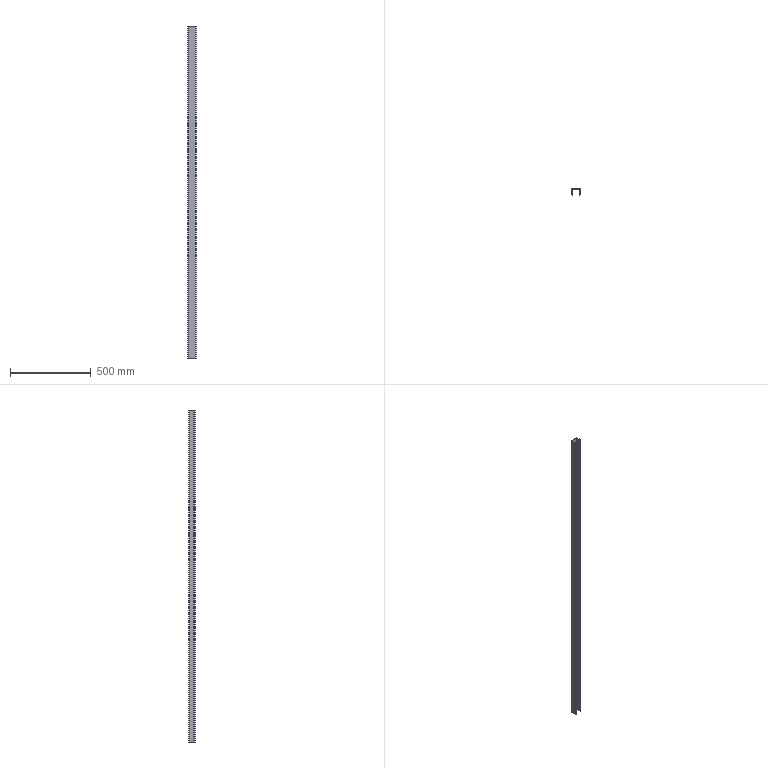Part | STEP file | 31E-01029QY25 | 1 solid | 28 faces | box 50 x 38.192 x 2050 mm | volume 337512 mm3 | plane 16 | cylinder 12 | commonest cylinder face diameters 1 x4 2 x4 4 x2 26 x2
STEP:
#1=CARTESIAN_POINT('',(27.993,8.298,1025.));
#2=VERTEX_POINT('',#1);
#3=CARTESIAN_POINT('',(32.281,3.187,1025.));
#4=VERTEX_POINT('',#3);
#5=CARTESIAN_POINT('',(30.137,5.743,1025.));
#6=DIRECTION('',(0.6428,-0.766,0.));
#7=VECTOR('',#6,1.);
#8=LINE('',#5,#7);
#9=EDGE_CURVE('',#2,#4,#8,.T.);
#10=ORIENTED_EDGE('',*,*,#9,.F.);
#11=CARTESIAN_POINT('',(27.993,8.298,-1025.));
#12=VERTEX_POINT('',#11);
#13=CARTESIAN_POINT('',(27.993,8.298,0.));
#14=DIRECTION('',(0.,0.,-1.));
#15=VECTOR('',#14,1.);
#16=LINE('',#13,#15);
#17=EDGE_CURVE('',#2,#12,#16,.T.);
#18=ORIENTED_EDGE('',*,*,#17,.T.);
#19=CARTESIAN_POINT('',(32.281,3.187,-1025.));
#20=VERTEX_POINT('',#19);
#21=CARTESIAN_POINT('',(30.137,5.743,-1025.));
#22=DIRECTION('',(0.6428,-0.766,0.));
#23=VECTOR('',#22,1.);
#24=LINE('',#21,#23);
#25=EDGE_CURVE('',#12,#20,#24,.T.);
#26=ORIENTED_EDGE('',*,*,#25,.T.);
#27=CARTESIAN_POINT('',(32.281,3.187,0.));
#28=DIRECTION('',(0.,0.,-1.));
#29=VECTOR('',#28,1.);
#30=LINE('',#27,#29);
#31=EDGE_CURVE('',#4,#20,#30,.T.);
#32=ORIENTED_EDGE('',*,*,#31,.F.);
#33=EDGE_LOOP('',(#10,#18,#26,#32));
#34=FACE_OUTER_BOUND('',#33,.T.);
#35=CARTESIAN_POINT('',(27.525,8.856,1025.));
#36=DIRECTION('',(0.766,0.6428,0.));
#37=DIRECTION('',(-0.6428,0.766,0.));
#38=AXIS2_PLACEMENT_3D('',#35,#36,#37);
#39=PLANE('',#38);
#40=ADVANCED_FACE('',(#34),#39,.F.);
#41=CARTESIAN_POINT('',(76.525,38.856,1025.));
#42=VERTEX_POINT('',#41);
#43=CARTESIAN_POINT('',(28.525,38.856,1025.));
#44=VERTEX_POINT('',#43);
#45=CARTESIAN_POINT('',(52.525,38.856,1025.));
#46=DIRECTION('',(-1.,0.,0.));
#47=VECTOR('',#46,1.);
#48=LINE('',#45,#47);
#49=EDGE_CURVE('',#42,#44,#48,.T.);
#50=ORIENTED_EDGE('',*,*,#49,.T.);
#51=CARTESIAN_POINT('',(27.525,37.856,1025.));
#52=VERTEX_POINT('',#51);
#53=CARTESIAN_POINT('',(28.525,37.856,1025.));
#54=DIRECTION('',(0.,0.,1.));
#55=AXIS2_PLACEMENT_3D('',#53,#54,$);
#56=CIRCLE('',#55,1.);
#57=EDGE_CURVE('',#44,#52,#56,.T.);
#58=ORIENTED_EDGE('',*,*,#57,.T.);
#59=CARTESIAN_POINT('',(27.525,9.584,1025.));
#60=VERTEX_POINT('',#59);
#61=CARTESIAN_POINT('',(27.525,23.72,1025.));
#62=DIRECTION('',(0.,-1.,0.));
#63=VECTOR('',#62,1.);
#64=LINE('',#61,#63);
#65=EDGE_CURVE('',#52,#60,#64,.T.);
#66=ORIENTED_EDGE('',*,*,#65,.T.);
#67=CARTESIAN_POINT('',(29.525,9.584,1025.));
#68=DIRECTION('',(0.,0.,1.));
#69=AXIS2_PLACEMENT_3D('',#67,#68,$);
#70=CIRCLE('',#69,2.);
#71=EDGE_CURVE('',#60,#2,#70,.T.);
#72=ORIENTED_EDGE('',*,*,#71,.T.);
#73=ORIENTED_EDGE('',*,*,#9,.T.);
#74=CARTESIAN_POINT('',(28.342,2.493,1025.));
#75=VERTEX_POINT('',#74);
#76=CARTESIAN_POINT('',(30.312,2.84,1025.));
#77=DIRECTION('',(-0.9848,-0.1736,0.));
#78=VECTOR('',#77,1.);
#79=LINE('',#76,#78);
#80=EDGE_CURVE('',#4,#75,#79,.T.);
#81=ORIENTED_EDGE('',*,*,#80,.T.);
#82=CARTESIAN_POINT('',(32.653,0.6877,1025.));
#83=VERTEX_POINT('',#82);
#84=CARTESIAN_POINT('',(35.437,13.386,1025.));
#85=DIRECTION('',(0.,0.,1.));
#86=AXIS2_PLACEMENT_3D('',#84,#85,$);
#87=CIRCLE('',#86,13.);
#88=EDGE_CURVE('',#75,#83,#87,.T.);
#89=ORIENTED_EDGE('',*,*,#88,.T.);
#90=CARTESIAN_POINT('',(33.867,1.665,1025.));
#91=VERTEX_POINT('',#90);
#92=CARTESIAN_POINT('',(32.867,1.665,1025.));
#93=DIRECTION('',(0.,0.,1.));
#94=AXIS2_PLACEMENT_3D('',#92,#93,$);
#95=CIRCLE('',#94,1.);
#96=EDGE_CURVE('',#83,#91,#95,.T.);
#97=ORIENTED_EDGE('',*,*,#96,.T.);
#98=CARTESIAN_POINT('',(33.867,2.983,1025.));
#99=VERTEX_POINT('',#98);
#100=CARTESIAN_POINT('',(33.867,2.324,1025.));
#101=DIRECTION('',(0.,1.,0.));
#102=VECTOR('',#101,1.);
#103=LINE('',#100,#102);
#104=EDGE_CURVE('',#91,#99,#103,.T.);
#105=ORIENTED_EDGE('',*,*,#104,.T.);
#106=CARTESIAN_POINT('',(33.75,3.304,1025.));
#107=VERTEX_POINT('',#106);
#108=CARTESIAN_POINT('',(33.367,2.983,1025.));
#109=DIRECTION('',(0.,0.,1.));
#110=AXIS2_PLACEMENT_3D('',#108,#109,$);
#111=CIRCLE('',#110,0.5);
#112=EDGE_CURVE('',#99,#107,#111,.T.);
#113=ORIENTED_EDGE('',*,*,#112,.T.);
#114=CARTESIAN_POINT('',(28.725,9.293,1025.));
#115=VERTEX_POINT('',#114);
#116=CARTESIAN_POINT('',(31.237,6.298,1025.));
#117=DIRECTION('',(-0.6428,0.766,0.));
#118=VECTOR('',#117,1.);
#119=LINE('',#116,#118);
#120=EDGE_CURVE('',#107,#115,#119,.T.);
#121=ORIENTED_EDGE('',*,*,#120,.T.);
#122=CARTESIAN_POINT('',(28.725,37.156,1025.));
#123=VERTEX_POINT('',#122);
#124=CARTESIAN_POINT('',(28.725,23.225,1025.));
#125=DIRECTION('',(0.,1.,0.));
#126=VECTOR('',#125,1.);
#127=LINE('',#124,#126);
#128=EDGE_CURVE('',#115,#123,#127,.T.);
#129=ORIENTED_EDGE('',*,*,#128,.T.);
#130=CARTESIAN_POINT('',(29.225,37.656,1025.));
#131=VERTEX_POINT('',#130);
#132=CARTESIAN_POINT('',(28.725,37.156,1025.));
#133=CARTESIAN_POINT('',(28.725,37.219,1025.));
#134=CARTESIAN_POINT('',(28.735,37.282,1025.));
#135=CARTESIAN_POINT('',(28.754,37.343,1025.));
#136=CARTESIAN_POINT('',(28.812,37.456,1025.));
#137=CARTESIAN_POINT('',(28.902,37.546,1025.));
#138=CARTESIAN_POINT('',(28.954,37.583,1025.));
#139=CARTESIAN_POINT('',(29.039,37.627,1025.));
#140=CARTESIAN_POINT('',(29.131,37.649,1025.));
#141=CARTESIAN_POINT('',(29.162,37.654,1025.));
#142=CARTESIAN_POINT('',(29.193,37.656,1025.));
#143=CARTESIAN_POINT('',(29.225,37.656,1025.));
#144=B_SPLINE_CURVE_WITH_KNOTS('',5,(#132,#133,#134,#135,#136,#137,#138,#139,#140,#141,#142,#143),.UNSPECIFIED.,.F.,.U.,(6,3,3,6),(0.,0.4443,0.8886,1.11),.UNSPECIFIED.);
#145=EDGE_CURVE('',#123,#131,#144,.T.);
#146=ORIENTED_EDGE('',*,*,#145,.T.);
#147=CARTESIAN_POINT('',(75.825,37.656,1025.));
#148=VERTEX_POINT('',#147);
#149=CARTESIAN_POINT('',(52.525,37.656,1025.));
#150=DIRECTION('',(1.,0.,0.));
#151=VECTOR('',#150,1.);
#152=LINE('',#149,#151);
#153=EDGE_CURVE('',#131,#148,#152,.T.);
#154=ORIENTED_EDGE('',*,*,#153,.T.);
#155=CARTESIAN_POINT('',(76.325,37.156,1025.));
#156=VERTEX_POINT('',#155);
#157=CARTESIAN_POINT('',(75.825,37.656,1025.));
#158=CARTESIAN_POINT('',(75.888,37.656,1025.));
#159=CARTESIAN_POINT('',(75.95,37.646,1025.));
#160=CARTESIAN_POINT('',(76.011,37.627,1025.));
#161=CARTESIAN_POINT('',(76.124,37.569,1025.));
#162=CARTESIAN_POINT('',(76.214,37.479,1025.));
#163=CARTESIAN_POINT('',(76.252,37.427,1025.));
#164=CARTESIAN_POINT('',(76.295,37.342,1025.));
#165=CARTESIAN_POINT('',(76.317,37.25,1025.));
#166=CARTESIAN_POINT('',(76.322,37.219,1025.));
#167=CARTESIAN_POINT('',(76.325,37.187,1025.));
#168=CARTESIAN_POINT('',(76.325,37.156,1025.));
#169=B_SPLINE_CURVE_WITH_KNOTS('',5,(#157,#158,#159,#160,#161,#162,#163,#164,#165,#166,#167,#168),.UNSPECIFIED.,.F.,.U.,(6,3,3,6),(0.,0.4443,0.8886,1.11),.UNSPECIFIED.);
#170=EDGE_CURVE('',#148,#156,#169,.T.);
#171=ORIENTED_EDGE('',*,*,#170,.T.);
#172=CARTESIAN_POINT('',(76.325,9.293,1025.));
#173=VERTEX_POINT('',#172);
#174=CARTESIAN_POINT('',(76.325,23.225,1025.));
#175=DIRECTION('',(0.,-1.,0.));
#176=VECTOR('',#175,1.);
#177=LINE('',#174,#176);
#178=EDGE_CURVE('',#156,#173,#177,.T.);
#179=ORIENTED_EDGE('',*,*,#178,.T.);
#180=CARTESIAN_POINT('',(71.299,3.304,1025.));
#181=VERTEX_POINT('',#180);
#182=CARTESIAN_POINT('',(73.812,6.298,1025.));
#183=DIRECTION('',(-0.6428,-0.766,0.));
#184=VECTOR('',#183,1.);
#185=LINE('',#182,#184);
#186=EDGE_CURVE('',#173,#181,#185,.T.);
#187=ORIENTED_EDGE('',*,*,#186,.T.);
#188=CARTESIAN_POINT('',(71.182,2.983,1025.));
#189=VERTEX_POINT('',#188);
#190=CARTESIAN_POINT('',(71.682,2.983,1025.));
#191=DIRECTION('',(0.,0.,1.));
#192=AXIS2_PLACEMENT_3D('',#190,#191,$);
#193=CIRCLE('',#192,0.5);
#194=EDGE_CURVE('',#181,#189,#193,.T.);
#195=ORIENTED_EDGE('',*,*,#194,.T.);
#196=CARTESIAN_POINT('',(71.182,1.665,1025.));
#197=VERTEX_POINT('',#196);
#198=CARTESIAN_POINT('',(71.182,2.324,1025.));
#199=DIRECTION('',(0.,-1.,0.));
#200=VECTOR('',#199,1.);
#201=LINE('',#198,#200);
#202=EDGE_CURVE('',#189,#197,#201,.T.);
#203=ORIENTED_EDGE('',*,*,#202,.T.);
#204=CARTESIAN_POINT('',(72.397,0.6877,1025.));
#205=VERTEX_POINT('',#204);
#206=CARTESIAN_POINT('',(72.182,1.665,1025.));
#207=DIRECTION('',(0.,0.,1.));
#208=AXIS2_PLACEMENT_3D('',#206,#207,$);
#209=CIRCLE('',#208,1.);
#210=EDGE_CURVE('',#197,#205,#209,.T.);
#211=ORIENTED_EDGE('',*,*,#210,.T.);
#212=CARTESIAN_POINT('',(76.707,2.493,1025.));
#213=VERTEX_POINT('',#212);
#214=CARTESIAN_POINT('',(69.613,13.386,1025.));
#215=DIRECTION('',(0.,0.,1.));
#216=AXIS2_PLACEMENT_3D('',#214,#215,$);
#217=CIRCLE('',#216,13.);
#218=EDGE_CURVE('',#205,#213,#217,.T.);
#219=ORIENTED_EDGE('',*,*,#218,.T.);
#220=CARTESIAN_POINT('',(72.768,3.187,1025.));
#221=VERTEX_POINT('',#220);
#222=CARTESIAN_POINT('',(74.738,2.84,1025.));
#223=DIRECTION('',(-0.9848,0.1736,0.));
#224=VECTOR('',#223,1.);
#225=LINE('',#222,#224);
#226=EDGE_CURVE('',#213,#221,#225,.T.);
#227=ORIENTED_EDGE('',*,*,#226,.T.);
#228=CARTESIAN_POINT('',(77.057,8.298,1025.));
#229=VERTEX_POINT('',#228);
#230=CARTESIAN_POINT('',(74.912,5.743,1025.));
#231=DIRECTION('',(0.6428,0.766,0.));
#232=VECTOR('',#231,1.);
#233=LINE('',#230,#232);
#234=EDGE_CURVE('',#221,#229,#233,.T.);
#235=ORIENTED_EDGE('',*,*,#234,.T.);
#236=CARTESIAN_POINT('',(77.525,9.584,1025.));
#237=VERTEX_POINT('',#236);
#238=CARTESIAN_POINT('',(75.525,9.584,1025.));
#239=DIRECTION('',(0.,0.,1.));
#240=AXIS2_PLACEMENT_3D('',#238,#239,$);
#241=CIRCLE('',#240,2.);
#242=EDGE_CURVE('',#229,#237,#241,.T.);
#243=ORIENTED_EDGE('',*,*,#242,.T.);
#244=CARTESIAN_POINT('',(77.525,37.856,1025.));
#245=VERTEX_POINT('',#244);
#246=CARTESIAN_POINT('',(77.525,23.72,1025.));
#247=DIRECTION('',(0.,1.,0.));
#248=VECTOR('',#247,1.);
#249=LINE('',#246,#248);
#250=EDGE_CURVE('',#237,#245,#249,.T.);
#251=ORIENTED_EDGE('',*,*,#250,.T.);
#252=CARTESIAN_POINT('',(76.525,37.856,1025.));
#253=DIRECTION('',(0.,0.,1.));
#254=AXIS2_PLACEMENT_3D('',#252,#253,$);
#255=CIRCLE('',#254,1.);
#256=EDGE_CURVE('',#245,#42,#255,.T.);
#257=ORIENTED_EDGE('',*,*,#256,.T.);
#258=EDGE_LOOP('',(#50,#58,#66,#72,#73,#81,#89,#97,#105,#113,#121,#129,#146,#154,#171,#179,#187,#195,#203,#211,#219,#227,#235,#243,#251,#257));
#259=FACE_OUTER_BOUND('',#258,.T.);
#260=CARTESIAN_POINT('',(35.437,13.386,1025.));
#261=DIRECTION('',(0.,0.,1.));
#262=DIRECTION('',(1.,0.,0.));
#263=AXIS2_PLACEMENT_3D('',#260,#261,#262);
#264=PLANE('',#263);
#265=ADVANCED_FACE('',(#259),#264,.T.);
#266=ORIENTED_EDGE('',*,*,#71,.F.);
#267=CARTESIAN_POINT('',(27.525,9.584,-1025.));
#268=VERTEX_POINT('',#267);
#269=CARTESIAN_POINT('',(27.525,9.584,1025.));
#270=DIRECTION('',(0.,0.,-1.));
#271=VECTOR('',#270,1.);
#272=LINE('',#269,#271);
#273=EDGE_CURVE('',#268,#60,#272,.F.);
#274=ORIENTED_EDGE('',*,*,#273,.F.);
#275=CARTESIAN_POINT('',(29.525,9.584,-1025.));
#276=DIRECTION('',(0.,0.,-1.));
#277=AXIS2_PLACEMENT_3D('',#275,#276,$);
#278=CIRCLE('',#277,2.);
#279=EDGE_CURVE('',#12,#268,#278,.T.);
#280=ORIENTED_EDGE('',*,*,#279,.F.);
#281=ORIENTED_EDGE('',*,*,#17,.F.);
#282=EDGE_LOOP('',(#266,#274,#280,#281));
#283=FACE_OUTER_BOUND('',#282,.T.);
#284=CARTESIAN_POINT('',(29.525,9.584,1025.));
#285=DIRECTION('',(0.,0.,-1.));
#286=DIRECTION('',(1.,0.,0.));
#287=AXIS2_PLACEMENT_3D('',#284,#285,#286);
#288=CYLINDRICAL_SURFACE('',#287,2.);
#289=ADVANCED_FACE('',(#283),#288,.T.);
#290=CARTESIAN_POINT('',(27.525,37.856,-1025.));
#291=VERTEX_POINT('',#290);
#292=CARTESIAN_POINT('',(28.525,38.856,-1025.));
#293=VERTEX_POINT('',#292);
#294=CARTESIAN_POINT('',(27.525,37.856,-1025.));
#295=CARTESIAN_POINT('',(27.525,37.954,-1025.));
#296=CARTESIAN_POINT('',(27.537,38.052,-1025.));
#297=CARTESIAN_POINT('',(27.561,38.148,-1025.));
#298=CARTESIAN_POINT('',(27.632,38.332,-1025.));
#299=CARTESIAN_POINT('',(27.745,38.494,-1025.));
#300=CARTESIAN_POINT('',(27.812,38.567,-1025.));
#301=CARTESIAN_POINT('',(27.961,38.696,-1025.));
#302=CARTESIAN_POINT('',(28.137,38.786,-1025.));
#303=CARTESIAN_POINT('',(28.23,38.819,-1025.));
#304=CARTESIAN_POINT('',(28.346,38.846,-1025.));
#305=CARTESIAN_POINT('',(28.464,38.855,-1025.));
#306=CARTESIAN_POINT('',(28.484,38.856,-1025.));
#307=CARTESIAN_POINT('',(28.505,38.856,-1025.));
#308=CARTESIAN_POINT('',(28.525,38.856,-1025.));
#309=B_SPLINE_CURVE_WITH_KNOTS('',5,(#294,#295,#296,#297,#298,#299,#300,#301,#302,#303,#304,#305,#306,#307,#308),.UNSPECIFIED.,.F.,.U.,(6,3,3,3,6),(0.,0.6928,1.386,2.078,2.221),.UNSPECIFIED.);
#310=EDGE_CURVE('',#291,#293,#309,.T.);
#311=ORIENTED_EDGE('',*,*,#310,.T.);
#312=CARTESIAN_POINT('',(76.525,38.856,-1025.));
#313=VERTEX_POINT('',#312);
#314=CARTESIAN_POINT('',(52.525,38.856,-1025.));
#315=DIRECTION('',(-1.,0.,0.));
#316=VECTOR('',#315,1.);
#317=LINE('',#314,#316);
#318=EDGE_CURVE('',#313,#293,#317,.T.);
#319=ORIENTED_EDGE('',*,*,#318,.F.);
#320=CARTESIAN_POINT('',(77.525,37.856,-1025.));
#321=VERTEX_POINT('',#320);
#322=CARTESIAN_POINT('',(76.525,38.856,-1025.));
#323=CARTESIAN_POINT('',(76.623,38.856,-1025.));
#324=CARTESIAN_POINT('',(76.721,38.844,-1025.));
#325=CARTESIAN_POINT('',(76.817,38.82,-1025.));
#326=CARTESIAN_POINT('',(77.001,38.749,-1025.));
#327=CARTESIAN_POINT('',(77.163,38.636,-1025.));
#328=CARTESIAN_POINT('',(77.236,38.569,-1025.));
#329=CARTESIAN_POINT('',(77.365,38.42,-1025.));
#330=CARTESIAN_POINT('',(77.454,38.244,-1025.));
#331=CARTESIAN_POINT('',(77.488,38.151,-1025.));
#332=CARTESIAN_POINT('',(77.514,38.035,-1025.));
#333=CARTESIAN_POINT('',(77.523,37.917,-1025.));
#334=CARTESIAN_POINT('',(77.524,37.897,-1025.));
#335=CARTESIAN_POINT('',(77.525,37.876,-1025.));
#336=CARTESIAN_POINT('',(77.525,37.856,-1025.));
#337=B_SPLINE_CURVE_WITH_KNOTS('',5,(#322,#323,#324,#325,#326,#327,#328,#329,#330,#331,#332,#333,#334,#335,#336),.UNSPECIFIED.,.F.,.U.,(6,3,3,3,6),(0.,0.6928,1.386,2.078,2.221),.UNSPECIFIED.);
#338=EDGE_CURVE('',#313,#321,#337,.T.);
#339=ORIENTED_EDGE('',*,*,#338,.T.);
#340=CARTESIAN_POINT('',(77.525,9.584,-1025.));
#341=VERTEX_POINT('',#340);
#342=CARTESIAN_POINT('',(77.525,23.72,-1025.));
#343=DIRECTION('',(0.,1.,0.));
#344=VECTOR('',#343,1.);
#345=LINE('',#342,#344);
#346=EDGE_CURVE('',#341,#321,#345,.T.);
#347=ORIENTED_EDGE('',*,*,#346,.F.);
#348=CARTESIAN_POINT('',(77.057,8.298,-1025.));
#349=VERTEX_POINT('',#348);
#350=CARTESIAN_POINT('',(77.525,9.584,-1025.));
#351=CARTESIAN_POINT('',(77.525,9.361,-1025.));
#352=CARTESIAN_POINT('',(77.494,9.137,-1025.));
#353=CARTESIAN_POINT('',(77.431,8.92,-1025.));
#354=CARTESIAN_POINT('',(77.316,8.662,-1025.));
#355=CARTESIAN_POINT('',(77.16,8.431,-1025.));
#356=CARTESIAN_POINT('',(77.127,8.385,-1025.));
#357=CARTESIAN_POINT('',(77.093,8.341,-1025.));
#358=CARTESIAN_POINT('',(77.057,8.298,-1025.));
#359=B_SPLINE_CURVE_WITH_KNOTS('',5,(#350,#351,#352,#353,#354,#355,#356,#357,#358),.UNSPECIFIED.,.F.,.U.,(6,3,6),(0.,1.58,1.974),.UNSPECIFIED.);
#360=EDGE_CURVE('',#341,#349,#359,.T.);
#361=ORIENTED_EDGE('',*,*,#360,.T.);
#362=CARTESIAN_POINT('',(72.768,3.187,-1025.));
#363=VERTEX_POINT('',#362);
#364=CARTESIAN_POINT('',(74.912,5.743,-1025.));
#365=DIRECTION('',(0.6428,0.766,0.));
#366=VECTOR('',#365,1.);
#367=LINE('',#364,#366);
#368=EDGE_CURVE('',#363,#349,#367,.T.);
#369=ORIENTED_EDGE('',*,*,#368,.F.);
#370=CARTESIAN_POINT('',(76.707,2.493,-1025.));
#371=VERTEX_POINT('',#370);
#372=CARTESIAN_POINT('',(74.738,2.84,-1025.));
#373=DIRECTION('',(-0.9848,0.1736,0.));
#374=VECTOR('',#373,1.);
#375=LINE('',#372,#374);
#376=EDGE_CURVE('',#371,#363,#375,.T.);
#377=ORIENTED_EDGE('',*,*,#376,.F.);
#378=CARTESIAN_POINT('',(72.397,0.6877,-1025.));
#379=VERTEX_POINT('',#378);
#380=CARTESIAN_POINT('',(69.613,13.386,-1025.));
#381=DIRECTION('',(0.,0.,1.));
#382=AXIS2_PLACEMENT_3D('',#380,#381,$);
#383=CIRCLE('',#382,13.);
#384=EDGE_CURVE('',#379,#371,#383,.T.);
#385=ORIENTED_EDGE('',*,*,#384,.F.);
#386=CARTESIAN_POINT('',(71.182,1.665,-1025.));
#387=VERTEX_POINT('',#386);
#388=CARTESIAN_POINT('',(72.182,1.665,-1025.));
#389=DIRECTION('',(0.,0.,1.));
#390=AXIS2_PLACEMENT_3D('',#388,#389,$);
#391=CIRCLE('',#390,1.);
#392=EDGE_CURVE('',#387,#379,#391,.T.);
#393=ORIENTED_EDGE('',*,*,#392,.F.);
#394=CARTESIAN_POINT('',(71.182,2.983,-1025.));
#395=VERTEX_POINT('',#394);
#396=CARTESIAN_POINT('',(71.182,2.324,-1025.));
#397=DIRECTION('',(0.,-1.,0.));
#398=VECTOR('',#397,1.);
#399=LINE('',#396,#398);
#400=EDGE_CURVE('',#395,#387,#399,.T.);
#401=ORIENTED_EDGE('',*,*,#400,.F.);
#402=CARTESIAN_POINT('',(71.299,3.304,-1025.));
#403=VERTEX_POINT('',#402);
#404=CARTESIAN_POINT('',(71.182,2.983,-1025.));
#405=CARTESIAN_POINT('',(71.182,3.038,-1025.));
#406=CARTESIAN_POINT('',(71.19,3.094,-1025.));
#407=CARTESIAN_POINT('',(71.206,3.149,-1025.));
#408=CARTESIAN_POINT('',(71.235,3.213,-1025.));
#409=CARTESIAN_POINT('',(71.274,3.271,-1025.));
#410=CARTESIAN_POINT('',(71.282,3.282,-1025.));
#411=CARTESIAN_POINT('',(71.29,3.293,-1025.));
#412=CARTESIAN_POINT('',(71.299,3.304,-1025.));
#413=B_SPLINE_CURVE_WITH_KNOTS('',5,(#404,#405,#406,#407,#408,#409,#410,#411,#412),.UNSPECIFIED.,.F.,.U.,(6,3,6),(0.,0.3949,0.4936),.UNSPECIFIED.);
#414=EDGE_CURVE('',#395,#403,#413,.T.);
#415=ORIENTED_EDGE('',*,*,#414,.T.);
#416=CARTESIAN_POINT('',(76.325,9.293,-1025.));
#417=VERTEX_POINT('',#416);
#418=CARTESIAN_POINT('',(73.812,6.298,-1025.));
#419=DIRECTION('',(-0.6428,-0.766,0.));
#420=VECTOR('',#419,1.);
#421=LINE('',#418,#420);
#422=EDGE_CURVE('',#417,#403,#421,.T.);
#423=ORIENTED_EDGE('',*,*,#422,.F.);
#424=CARTESIAN_POINT('',(76.325,37.156,-1025.));
#425=VERTEX_POINT('',#424);
#426=CARTESIAN_POINT('',(76.325,23.225,-1025.));
#427=DIRECTION('',(0.,-1.,0.));
#428=VECTOR('',#427,1.);
#429=LINE('',#426,#428);
#430=EDGE_CURVE('',#425,#417,#429,.T.);
#431=ORIENTED_EDGE('',*,*,#430,.F.);
#432=CARTESIAN_POINT('',(75.825,37.656,-1025.));
#433=VERTEX_POINT('',#432);
#434=CARTESIAN_POINT('',(75.825,37.156,-1025.));
#435=DIRECTION('',(0.,0.,1.));
#436=AXIS2_PLACEMENT_3D('',#434,#435,$);
#437=CIRCLE('',#436,0.5);
#438=EDGE_CURVE('',#425,#433,#437,.T.);
#439=ORIENTED_EDGE('',*,*,#438,.T.);
#440=CARTESIAN_POINT('',(29.225,37.656,-1025.));
#441=VERTEX_POINT('',#440);
#442=CARTESIAN_POINT('',(52.525,37.656,-1025.));
#443=DIRECTION('',(1.,0.,0.));
#444=VECTOR('',#443,1.);
#445=LINE('',#442,#444);
#446=EDGE_CURVE('',#441,#433,#445,.T.);
#447=ORIENTED_EDGE('',*,*,#446,.F.);
#448=CARTESIAN_POINT('',(28.725,37.156,-1025.));
#449=VERTEX_POINT('',#448);
#450=CARTESIAN_POINT('',(29.225,37.156,-1025.));
#451=DIRECTION('',(0.,0.,1.));
#452=AXIS2_PLACEMENT_3D('',#450,#451,$);
#453=CIRCLE('',#452,0.5);
#454=EDGE_CURVE('',#441,#449,#453,.T.);
#455=ORIENTED_EDGE('',*,*,#454,.T.);
#456=CARTESIAN_POINT('',(28.725,9.293,-1025.));
#457=VERTEX_POINT('',#456);
#458=CARTESIAN_POINT('',(28.725,23.225,-1025.));
#459=DIRECTION('',(0.,1.,0.));
#460=VECTOR('',#459,1.);
#461=LINE('',#458,#460);
#462=EDGE_CURVE('',#457,#449,#461,.T.);
#463=ORIENTED_EDGE('',*,*,#462,.F.);
#464=CARTESIAN_POINT('',(33.75,3.304,-1025.));
#465=VERTEX_POINT('',#464);
#466=CARTESIAN_POINT('',(31.237,6.298,-1025.));
#467=DIRECTION('',(-0.6428,0.766,0.));
#468=VECTOR('',#467,1.);
#469=LINE('',#466,#468);
#470=EDGE_CURVE('',#465,#457,#469,.T.);
#471=ORIENTED_EDGE('',*,*,#470,.F.);
#472=CARTESIAN_POINT('',(33.867,2.983,-1025.));
#473=VERTEX_POINT('',#472);
#474=CARTESIAN_POINT('',(33.75,3.304,-1025.));
#475=CARTESIAN_POINT('',(33.786,3.261,-1025.));
#476=CARTESIAN_POINT('',(33.816,3.213,-1025.));
#477=CARTESIAN_POINT('',(33.839,3.162,-1025.));
#478=CARTESIAN_POINT('',(33.858,3.094,-1025.));
#479=CARTESIAN_POINT('',(33.866,3.024,-1025.));
#480=CARTESIAN_POINT('',(33.867,3.01,-1025.));
#481=CARTESIAN_POINT('',(33.867,2.997,-1025.));
#482=CARTESIAN_POINT('',(33.867,2.983,-1025.));
#483=B_SPLINE_CURVE_WITH_KNOTS('',5,(#474,#475,#476,#477,#478,#479,#480,#481,#482),.UNSPECIFIED.,.F.,.U.,(6,3,6),(0.,0.3949,0.4936),.UNSPECIFIED.);
#484=EDGE_CURVE('',#465,#473,#483,.T.);
#485=ORIENTED_EDGE('',*,*,#484,.T.);
#486=CARTESIAN_POINT('',(33.867,1.665,-1025.));
#487=VERTEX_POINT('',#486);
#488=CARTESIAN_POINT('',(33.867,2.324,-1025.));
#489=DIRECTION('',(0.,1.,0.));
#490=VECTOR('',#489,1.);
#491=LINE('',#488,#490);
#492=EDGE_CURVE('',#487,#473,#491,.T.);
#493=ORIENTED_EDGE('',*,*,#492,.F.);
#494=CARTESIAN_POINT('',(32.653,0.6877,-1025.));
#495=VERTEX_POINT('',#494);
#496=CARTESIAN_POINT('',(32.867,1.665,-1025.));
#497=DIRECTION('',(0.,0.,1.));
#498=AXIS2_PLACEMENT_3D('',#496,#497,$);
#499=CIRCLE('',#498,1.);
#500=EDGE_CURVE('',#495,#487,#499,.T.);
#501=ORIENTED_EDGE('',*,*,#500,.F.);
#502=CARTESIAN_POINT('',(28.342,2.493,-1025.));
#503=VERTEX_POINT('',#502);
#504=CARTESIAN_POINT('',(35.437,13.386,-1025.));
#505=DIRECTION('',(0.,0.,1.));
#506=AXIS2_PLACEMENT_3D('',#504,#505,$);
#507=CIRCLE('',#506,13.);
#508=EDGE_CURVE('',#503,#495,#507,.T.);
#509=ORIENTED_EDGE('',*,*,#508,.F.);
#510=CARTESIAN_POINT('',(30.312,2.84,-1025.));
#511=DIRECTION('',(-0.9848,-0.1736,0.));
#512=VECTOR('',#511,1.);
#513=LINE('',#510,#512);
#514=EDGE_CURVE('',#20,#503,#513,.T.);
#515=ORIENTED_EDGE('',*,*,#514,.F.);
#516=ORIENTED_EDGE('',*,*,#25,.F.);
#517=ORIENTED_EDGE('',*,*,#279,.T.);
#518=CARTESIAN_POINT('',(27.525,23.72,-1025.));
#519=DIRECTION('',(0.,-1.,0.));
#520=VECTOR('',#519,1.);
#521=LINE('',#518,#520);
#522=EDGE_CURVE('',#291,#268,#521,.T.);
#523=ORIENTED_EDGE('',*,*,#522,.F.);
#524=EDGE_LOOP('',(#311,#319,#339,#347,#361,#369,#377,#385,#393,#401,#415,#423,#431,#439,#447,#455,#463,#471,#485,#493,#501,#509,#515,#516,#517,#523));
#525=FACE_OUTER_BOUND('',#524,.T.);
#526=CARTESIAN_POINT('',(35.437,13.386,-1025.));
#527=DIRECTION('',(0.,0.,1.));
#528=DIRECTION('',(1.,0.,0.));
#529=AXIS2_PLACEMENT_3D('',#526,#527,#528);
#530=PLANE('',#529);
#531=ADVANCED_FACE('',(#525),#530,.F.);
#532=ORIENTED_EDGE('',*,*,#514,.T.);
#533=CARTESIAN_POINT('',(28.342,2.493,0.));
#534=DIRECTION('',(0.,0.,-1.));
#535=VECTOR('',#534,1.);
#536=LINE('',#533,#535);
#537=EDGE_CURVE('',#75,#503,#536,.T.);
#538=ORIENTED_EDGE('',*,*,#537,.F.);
#539=ORIENTED_EDGE('',*,*,#80,.F.);
#540=ORIENTED_EDGE('',*,*,#31,.T.);
#541=EDGE_LOOP('',(#532,#538,#539,#540));
#542=FACE_OUTER_BOUND('',#541,.T.);
#543=CARTESIAN_POINT('',(32.281,3.187,1025.));
#544=DIRECTION('',(0.1736,-0.9848,0.));
#545=DIRECTION('',(0.9848,0.1736,0.));
#546=AXIS2_PLACEMENT_3D('',#543,#544,#545);
#547=PLANE('',#546);
#548=ADVANCED_FACE('',(#542),#547,.F.);
#549=ORIENTED_EDGE('',*,*,#318,.T.);
#550=CARTESIAN_POINT('',(28.525,38.856,0.));
#551=DIRECTION('',(0.,0.,1.));
#552=VECTOR('',#551,1.);
#553=LINE('',#550,#552);
#554=EDGE_CURVE('',#293,#44,#553,.T.);
#555=ORIENTED_EDGE('',*,*,#554,.T.);
#556=ORIENTED_EDGE('',*,*,#49,.F.);
#557=CARTESIAN_POINT('',(76.525,38.856,0.));
#558=DIRECTION('',(0.,0.,-1.));
#559=VECTOR('',#558,1.);
#560=LINE('',#557,#559);
#561=EDGE_CURVE('',#42,#313,#560,.T.);
#562=ORIENTED_EDGE('',*,*,#561,.T.);
#563=EDGE_LOOP('',(#549,#555,#556,#562));
#564=FACE_OUTER_BOUND('',#563,.T.);
#565=CARTESIAN_POINT('',(27.525,38.856,1025.));
#566=DIRECTION('',(0.,-1.,0.));
#567=DIRECTION('',(1.,0.,0.));
#568=AXIS2_PLACEMENT_3D('',#565,#566,#567);
#569=PLANE('',#568);
#570=ADVANCED_FACE('',(#564),#569,.F.);
#571=ORIENTED_EDGE('',*,*,#57,.F.);
#572=ORIENTED_EDGE('',*,*,#554,.F.);
#573=ORIENTED_EDGE('',*,*,#310,.F.);
#574=CARTESIAN_POINT('',(27.525,37.856,1025.));
#575=DIRECTION('',(0.,0.,-1.));
#576=VECTOR('',#575,1.);
#577=LINE('',#574,#576);
#578=EDGE_CURVE('',#52,#291,#577,.T.);
#579=ORIENTED_EDGE('',*,*,#578,.F.);
#580=EDGE_LOOP('',(#571,#572,#573,#579));
#581=FACE_OUTER_BOUND('',#580,.T.);
#582=CARTESIAN_POINT('',(28.525,37.856,1025.));
#583=DIRECTION('',(0.,0.,-1.));
#584=DIRECTION('',(-1.,0.,0.));
#585=AXIS2_PLACEMENT_3D('',#582,#583,#584);
#586=CYLINDRICAL_SURFACE('',#585,1.);
#587=ADVANCED_FACE('',(#581),#586,.T.);
#588=ORIENTED_EDGE('',*,*,#65,.F.);
#589=ORIENTED_EDGE('',*,*,#578,.T.);
#590=ORIENTED_EDGE('',*,*,#522,.T.);
#591=ORIENTED_EDGE('',*,*,#273,.T.);
#592=EDGE_LOOP('',(#588,#589,#590,#591));
#593=FACE_OUTER_BOUND('',#592,.T.);
#594=CARTESIAN_POINT('',(27.525,8.856,1025.));
#595=DIRECTION('',(1.,0.,0.));
#596=DIRECTION('',(0.,0.,-1.));
#597=AXIS2_PLACEMENT_3D('',#594,#595,#596);
#598=PLANE('',#597);
#599=ADVANCED_FACE('',(#593),#598,.F.);
#600=ORIENTED_EDGE('',*,*,#508,.T.);
#601=CARTESIAN_POINT('',(32.653,0.6877,1025.));
#602=DIRECTION('',(0.,0.,-1.));
#603=VECTOR('',#602,1.);
#604=LINE('',#601,#603);
#605=EDGE_CURVE('',#83,#495,#604,.T.);
#606=ORIENTED_EDGE('',*,*,#605,.F.);
#607=ORIENTED_EDGE('',*,*,#88,.F.);
#608=ORIENTED_EDGE('',*,*,#537,.T.);
#609=EDGE_LOOP('',(#600,#606,#607,#608));
#610=FACE_OUTER_BOUND('',#609,.T.);
#611=CARTESIAN_POINT('',(35.437,13.386,1025.));
#612=DIRECTION('',(0.,0.,-1.));
#613=DIRECTION('',(1.,0.,0.));
#614=AXIS2_PLACEMENT_3D('',#611,#612,#613);
#615=CYLINDRICAL_SURFACE('',#614,13.);
#616=ADVANCED_FACE('',(#610),#615,.T.);
#617=ORIENTED_EDGE('',*,*,#500,.T.);
#618=CARTESIAN_POINT('',(33.867,1.665,1025.));
#619=DIRECTION('',(0.,0.,-1.));
#620=VECTOR('',#619,1.);
#621=LINE('',#618,#620);
#622=EDGE_CURVE('',#91,#487,#621,.T.);
#623=ORIENTED_EDGE('',*,*,#622,.F.);
#624=ORIENTED_EDGE('',*,*,#96,.F.);
#625=ORIENTED_EDGE('',*,*,#605,.T.);
#626=EDGE_LOOP('',(#617,#623,#624,#625));
#627=FACE_OUTER_BOUND('',#626,.T.);
#628=CARTESIAN_POINT('',(32.867,1.665,1025.));
#629=DIRECTION('',(0.,0.,-1.));
#630=DIRECTION('',(1.,0.,0.));
#631=AXIS2_PLACEMENT_3D('',#628,#629,#630);
#632=CYLINDRICAL_SURFACE('',#631,1.);
#633=ADVANCED_FACE('',(#627),#632,.T.);
#634=ORIENTED_EDGE('',*,*,#492,.T.);
#635=CARTESIAN_POINT('',(33.867,2.983,0.));
#636=DIRECTION('',(0.,0.,1.));
#637=VECTOR('',#636,1.);
#638=LINE('',#635,#637);
#639=EDGE_CURVE('',#473,#99,#638,.T.);
#640=ORIENTED_EDGE('',*,*,#639,.T.);
#641=ORIENTED_EDGE('',*,*,#104,.F.);
#642=ORIENTED_EDGE('',*,*,#622,.T.);
#643=EDGE_LOOP('',(#634,#640,#641,#642));
#644=FACE_OUTER_BOUND('',#643,.T.);
#645=CARTESIAN_POINT('',(33.867,1.665,1025.));
#646=DIRECTION('',(-1.,0.,0.));
#647=DIRECTION('',(0.,0.,1.));
#648=AXIS2_PLACEMENT_3D('',#645,#646,#647);
#649=PLANE('',#648);
#650=ADVANCED_FACE('',(#644),#649,.F.);
#651=ORIENTED_EDGE('',*,*,#112,.F.);
#652=ORIENTED_EDGE('',*,*,#639,.F.);
#653=ORIENTED_EDGE('',*,*,#484,.F.);
#654=CARTESIAN_POINT('',(33.75,3.304,1025.));
#655=DIRECTION('',(0.,0.,-1.));
#656=VECTOR('',#655,1.);
#657=LINE('',#654,#656);
#658=EDGE_CURVE('',#107,#465,#657,.T.);
#659=ORIENTED_EDGE('',*,*,#658,.F.);
#660=EDGE_LOOP('',(#651,#652,#653,#659));
#661=FACE_OUTER_BOUND('',#660,.T.);
#662=CARTESIAN_POINT('',(33.367,2.983,1025.));
#663=DIRECTION('',(0.,0.,-1.));
#664=DIRECTION('',(-1.,0.,0.));
#665=AXIS2_PLACEMENT_3D('',#662,#663,#664);
#666=CYLINDRICAL_SURFACE('',#665,0.5);
#667=ADVANCED_FACE('',(#661),#666,.T.);
#668=ORIENTED_EDGE('',*,*,#120,.F.);
#669=ORIENTED_EDGE('',*,*,#658,.T.);
#670=ORIENTED_EDGE('',*,*,#470,.T.);
#671=CARTESIAN_POINT('',(28.725,9.293,0.));
#672=DIRECTION('',(0.,0.,-1.));
#673=VECTOR('',#672,1.);
#674=LINE('',#671,#673);
#675=EDGE_CURVE('',#115,#457,#674,.T.);
#676=ORIENTED_EDGE('',*,*,#675,.F.);
#677=EDGE_LOOP('',(#668,#669,#670,#676));
#678=FACE_OUTER_BOUND('',#677,.T.);
#679=CARTESIAN_POINT('',(28.725,9.293,1025.));
#680=DIRECTION('',(-0.766,-0.6428,0.));
#681=DIRECTION('',(0.6428,-0.766,0.));
#682=AXIS2_PLACEMENT_3D('',#679,#680,#681);
#683=PLANE('',#682);
#684=ADVANCED_FACE('',(#678),#683,.F.);
#685=ORIENTED_EDGE('',*,*,#462,.T.);
#686=CARTESIAN_POINT('',(28.725,37.156,0.));
#687=DIRECTION('',(0.,0.,1.));
#688=VECTOR('',#687,1.);
#689=LINE('',#686,#688);
#690=EDGE_CURVE('',#449,#123,#689,.T.);
#691=ORIENTED_EDGE('',*,*,#690,.T.);
#692=ORIENTED_EDGE('',*,*,#128,.F.);
#693=ORIENTED_EDGE('',*,*,#675,.T.);
#694=EDGE_LOOP('',(#685,#691,#692,#693));
#695=FACE_OUTER_BOUND('',#694,.T.);
#696=CARTESIAN_POINT('',(28.725,9.293,1025.));
#697=DIRECTION('',(-1.,0.,0.));
#698=DIRECTION('',(0.,0.,1.));
#699=AXIS2_PLACEMENT_3D('',#696,#697,#698);
#700=PLANE('',#699);
#701=ADVANCED_FACE('',(#695),#700,.F.);
#702=ORIENTED_EDGE('',*,*,#145,.F.);
#703=ORIENTED_EDGE('',*,*,#690,.F.);
#704=ORIENTED_EDGE('',*,*,#454,.F.);
#705=CARTESIAN_POINT('',(29.225,37.656,1025.));
#706=DIRECTION('',(0.,0.,1.));
#707=VECTOR('',#706,1.);
#708=LINE('',#705,#707);
#709=EDGE_CURVE('',#131,#441,#708,.F.);
#710=ORIENTED_EDGE('',*,*,#709,.F.);
#711=EDGE_LOOP('',(#702,#703,#704,#710));
#712=FACE_OUTER_BOUND('',#711,.T.);
#713=CARTESIAN_POINT('',(29.225,37.156,1025.));
#714=DIRECTION('',(0.,0.,1.));
#715=DIRECTION('',(1.,0.,0.));
#716=AXIS2_PLACEMENT_3D('',#713,#714,#715);
#717=CYLINDRICAL_SURFACE('',#716,0.5);
#718=ADVANCED_FACE('',(#712),#717,.F.);
#719=ORIENTED_EDGE('',*,*,#446,.T.);
#720=CARTESIAN_POINT('',(75.825,37.656,0.));
#721=DIRECTION('',(0.,0.,1.));
#722=VECTOR('',#721,1.);
#723=LINE('',#720,#722);
#724=EDGE_CURVE('',#433,#148,#723,.T.);
#725=ORIENTED_EDGE('',*,*,#724,.T.);
#726=ORIENTED_EDGE('',*,*,#153,.F.);
#727=ORIENTED_EDGE('',*,*,#709,.T.);
#728=EDGE_LOOP('',(#719,#725,#726,#727));
#729=FACE_OUTER_BOUND('',#728,.T.);
#730=CARTESIAN_POINT('',(28.725,37.656,1025.));
#731=DIRECTION('',(0.,1.,0.));
#732=DIRECTION('',(-1.,0.,0.));
#733=AXIS2_PLACEMENT_3D('',#730,#731,#732);
#734=PLANE('',#733);
#735=ADVANCED_FACE('',(#729),#734,.F.);
#736=ORIENTED_EDGE('',*,*,#170,.F.);
#737=ORIENTED_EDGE('',*,*,#724,.F.);
#738=ORIENTED_EDGE('',*,*,#438,.F.);
#739=CARTESIAN_POINT('',(76.325,37.156,1025.));
#740=DIRECTION('',(0.,0.,1.));
#741=VECTOR('',#740,1.);
#742=LINE('',#739,#741);
#743=EDGE_CURVE('',#156,#425,#742,.F.);
#744=ORIENTED_EDGE('',*,*,#743,.F.);
#745=EDGE_LOOP('',(#736,#737,#738,#744));
#746=FACE_OUTER_BOUND('',#745,.T.);
#747=CARTESIAN_POINT('',(75.825,37.156,1025.));
#748=DIRECTION('',(0.,0.,1.));
#749=DIRECTION('',(1.,0.,0.));
#750=AXIS2_PLACEMENT_3D('',#747,#748,#749);
#751=CYLINDRICAL_SURFACE('',#750,0.5);
#752=ADVANCED_FACE('',(#746),#751,.F.);
#753=ORIENTED_EDGE('',*,*,#178,.F.);
#754=ORIENTED_EDGE('',*,*,#743,.T.);
#755=ORIENTED_EDGE('',*,*,#430,.T.);
#756=CARTESIAN_POINT('',(76.325,9.293,0.));
#757=DIRECTION('',(0.,0.,-1.));
#758=VECTOR('',#757,1.);
#759=LINE('',#756,#758);
#760=EDGE_CURVE('',#173,#417,#759,.T.);
#761=ORIENTED_EDGE('',*,*,#760,.F.);
#762=EDGE_LOOP('',(#753,#754,#755,#761));
#763=FACE_OUTER_BOUND('',#762,.T.);
#764=CARTESIAN_POINT('',(76.325,9.293,1025.));
#765=DIRECTION('',(1.,0.,0.));
#766=DIRECTION('',(0.,1.,0.));
#767=AXIS2_PLACEMENT_3D('',#764,#765,#766);
#768=PLANE('',#767);
#769=ADVANCED_FACE('',(#763),#768,.F.);
#770=ORIENTED_EDGE('',*,*,#422,.T.);
#771=CARTESIAN_POINT('',(71.299,3.304,0.));
#772=DIRECTION('',(0.,0.,1.));
#773=VECTOR('',#772,1.);
#774=LINE('',#771,#773);
#775=EDGE_CURVE('',#403,#181,#774,.T.);
#776=ORIENTED_EDGE('',*,*,#775,.T.);
#777=ORIENTED_EDGE('',*,*,#186,.F.);
#778=ORIENTED_EDGE('',*,*,#760,.T.);
#779=EDGE_LOOP('',(#770,#776,#777,#778));
#780=FACE_OUTER_BOUND('',#779,.T.);
#781=CARTESIAN_POINT('',(76.325,9.293,1025.));
#782=DIRECTION('',(0.766,-0.6428,0.));
#783=DIRECTION('',(0.6428,0.766,0.));
#784=AXIS2_PLACEMENT_3D('',#781,#782,#783);
#785=PLANE('',#784);
#786=ADVANCED_FACE('',(#780),#785,.F.);
#787=ORIENTED_EDGE('',*,*,#194,.F.);
#788=ORIENTED_EDGE('',*,*,#775,.F.);
#789=ORIENTED_EDGE('',*,*,#414,.F.);
#790=CARTESIAN_POINT('',(71.182,2.983,1025.));
#791=DIRECTION('',(0.,0.,-1.));
#792=VECTOR('',#791,1.);
#793=LINE('',#790,#792);
#794=EDGE_CURVE('',#189,#395,#793,.T.);
#795=ORIENTED_EDGE('',*,*,#794,.F.);
#796=EDGE_LOOP('',(#787,#788,#789,#795));
#797=FACE_OUTER_BOUND('',#796,.T.);
#798=CARTESIAN_POINT('',(71.682,2.983,1025.));
#799=DIRECTION('',(0.,0.,-1.));
#800=DIRECTION('',(-1.,0.,0.));
#801=AXIS2_PLACEMENT_3D('',#798,#799,#800);
#802=CYLINDRICAL_SURFACE('',#801,0.5);
#803=ADVANCED_FACE('',(#797),#802,.T.);
#804=ORIENTED_EDGE('',*,*,#202,.F.);
#805=ORIENTED_EDGE('',*,*,#794,.T.);
#806=ORIENTED_EDGE('',*,*,#400,.T.);
#807=CARTESIAN_POINT('',(71.182,1.665,0.));
#808=DIRECTION('',(0.,0.,-1.));
#809=VECTOR('',#808,1.);
#810=LINE('',#807,#809);
#811=EDGE_CURVE('',#197,#387,#810,.T.);
#812=ORIENTED_EDGE('',*,*,#811,.F.);
#813=EDGE_LOOP('',(#804,#805,#806,#812));
#814=FACE_OUTER_BOUND('',#813,.T.);
#815=CARTESIAN_POINT('',(71.182,1.665,1025.));
#816=DIRECTION('',(1.,0.,0.));
#817=DIRECTION('',(0.,0.,-1.));
#818=AXIS2_PLACEMENT_3D('',#815,#816,#817);
#819=PLANE('',#818);
#820=ADVANCED_FACE('',(#814),#819,.F.);
#821=ORIENTED_EDGE('',*,*,#392,.T.);
#822=CARTESIAN_POINT('',(72.397,0.6877,1025.));
#823=DIRECTION('',(0.,0.,-1.));
#824=VECTOR('',#823,1.);
#825=LINE('',#822,#824);
#826=EDGE_CURVE('',#205,#379,#825,.T.);
#827=ORIENTED_EDGE('',*,*,#826,.F.);
#828=ORIENTED_EDGE('',*,*,#210,.F.);
#829=ORIENTED_EDGE('',*,*,#811,.T.);
#830=EDGE_LOOP('',(#821,#827,#828,#829));
#831=FACE_OUTER_BOUND('',#830,.T.);
#832=CARTESIAN_POINT('',(72.182,1.665,1025.));
#833=DIRECTION('',(0.,0.,-1.));
#834=DIRECTION('',(1.,0.,0.));
#835=AXIS2_PLACEMENT_3D('',#832,#833,#834);
#836=CYLINDRICAL_SURFACE('',#835,1.);
#837=ADVANCED_FACE('',(#831),#836,.T.);
#838=ORIENTED_EDGE('',*,*,#384,.T.);
#839=CARTESIAN_POINT('',(76.707,2.493,1025.));
#840=DIRECTION('',(0.,0.,-1.));
#841=VECTOR('',#840,1.);
#842=LINE('',#839,#841);
#843=EDGE_CURVE('',#213,#371,#842,.T.);
#844=ORIENTED_EDGE('',*,*,#843,.F.);
#845=ORIENTED_EDGE('',*,*,#218,.F.);
#846=ORIENTED_EDGE('',*,*,#826,.T.);
#847=EDGE_LOOP('',(#838,#844,#845,#846));
#848=FACE_OUTER_BOUND('',#847,.T.);
#849=CARTESIAN_POINT('',(69.613,13.386,1025.));
#850=DIRECTION('',(0.,0.,-1.));
#851=DIRECTION('',(1.,0.,0.));
#852=AXIS2_PLACEMENT_3D('',#849,#850,#851);
#853=CYLINDRICAL_SURFACE('',#852,13.);
#854=ADVANCED_FACE('',(#848),#853,.T.);
#855=ORIENTED_EDGE('',*,*,#376,.T.);
#856=CARTESIAN_POINT('',(72.768,3.187,0.));
#857=DIRECTION('',(0.,0.,-1.));
#858=VECTOR('',#857,1.);
#859=LINE('',#856,#858);
#860=EDGE_CURVE('',#221,#363,#859,.T.);
#861=ORIENTED_EDGE('',*,*,#860,.F.);
#862=ORIENTED_EDGE('',*,*,#226,.F.);
#863=ORIENTED_EDGE('',*,*,#843,.T.);
#864=EDGE_LOOP('',(#855,#861,#862,#863));
#865=FACE_OUTER_BOUND('',#864,.T.);
#866=CARTESIAN_POINT('',(72.768,3.187,1025.));
#867=DIRECTION('',(-0.1736,-0.9848,0.));
#868=DIRECTION('',(0.9848,-0.1736,0.));
#869=AXIS2_PLACEMENT_3D('',#866,#867,#868);
#870=PLANE('',#869);
#871=ADVANCED_FACE('',(#865),#870,.F.);
#872=ORIENTED_EDGE('',*,*,#368,.T.);
#873=CARTESIAN_POINT('',(77.057,8.298,0.));
#874=DIRECTION('',(0.,0.,1.));
#875=VECTOR('',#874,1.);
#876=LINE('',#873,#875);
#877=EDGE_CURVE('',#349,#229,#876,.T.);
#878=ORIENTED_EDGE('',*,*,#877,.T.);
#879=ORIENTED_EDGE('',*,*,#234,.F.);
#880=ORIENTED_EDGE('',*,*,#860,.T.);
#881=EDGE_LOOP('',(#872,#878,#879,#880));
#882=FACE_OUTER_BOUND('',#881,.T.);
#883=CARTESIAN_POINT('',(77.525,8.856,1025.));
#884=DIRECTION('',(-0.766,0.6428,0.));
#885=DIRECTION('',(-0.6428,-0.766,0.));
#886=AXIS2_PLACEMENT_3D('',#883,#884,#885);
#887=PLANE('',#886);
#888=ADVANCED_FACE('',(#882),#887,.F.);
#889=ORIENTED_EDGE('',*,*,#242,.F.);
#890=ORIENTED_EDGE('',*,*,#877,.F.);
#891=ORIENTED_EDGE('',*,*,#360,.F.);
#892=CARTESIAN_POINT('',(77.525,9.584,1025.));
#893=DIRECTION('',(0.,0.,-1.));
#894=VECTOR('',#893,1.);
#895=LINE('',#892,#894);
#896=EDGE_CURVE('',#237,#341,#895,.T.);
#897=ORIENTED_EDGE('',*,*,#896,.F.);
#898=EDGE_LOOP('',(#889,#890,#891,#897));
#899=FACE_OUTER_BOUND('',#898,.T.);
#900=CARTESIAN_POINT('',(75.525,9.584,1025.));
#901=DIRECTION('',(0.,0.,-1.));
#902=DIRECTION('',(1.,0.,0.));
#903=AXIS2_PLACEMENT_3D('',#900,#901,#902);
#904=CYLINDRICAL_SURFACE('',#903,2.);
#905=ADVANCED_FACE('',(#899),#904,.T.);
#906=ORIENTED_EDGE('',*,*,#346,.T.);
#907=CARTESIAN_POINT('',(77.525,37.856,0.));
#908=DIRECTION('',(0.,0.,1.));
#909=VECTOR('',#908,1.);
#910=LINE('',#907,#909);
#911=EDGE_CURVE('',#321,#245,#910,.T.);
#912=ORIENTED_EDGE('',*,*,#911,.T.);
#913=ORIENTED_EDGE('',*,*,#250,.F.);
#914=ORIENTED_EDGE('',*,*,#896,.T.);
#915=EDGE_LOOP('',(#906,#912,#913,#914));
#916=FACE_OUTER_BOUND('',#915,.T.);
#917=CARTESIAN_POINT('',(77.525,8.856,1025.));
#918=DIRECTION('',(-1.,0.,0.));
#919=DIRECTION('',(0.,0.,1.));
#920=AXIS2_PLACEMENT_3D('',#917,#918,#919);
#921=PLANE('',#920);
#922=ADVANCED_FACE('',(#916),#921,.F.);
#923=ORIENTED_EDGE('',*,*,#256,.F.);
#924=ORIENTED_EDGE('',*,*,#911,.F.);
#925=ORIENTED_EDGE('',*,*,#338,.F.);
#926=ORIENTED_EDGE('',*,*,#561,.F.);
#927=EDGE_LOOP('',(#923,#924,#925,#926));
#928=FACE_OUTER_BOUND('',#927,.T.);
#929=CARTESIAN_POINT('',(76.525,37.856,1025.));
#930=DIRECTION('',(0.,0.,-1.));
#931=DIRECTION('',(-1.,0.,0.));
#932=AXIS2_PLACEMENT_3D('',#929,#930,#931);
#933=CYLINDRICAL_SURFACE('',#932,1.);
#934=ADVANCED_FACE('',(#928),#933,.T.);
#935=CLOSED_SHELL('',(#40,#265,#289,#531,#548,#570,#587,#599,#616,#633,#650,#667,#684,#701,#718,#735,#752,#769,#786,#803,#820,#837,#854,#871,#888,#905,#922,#934));
#936=MANIFOLD_SOLID_BREP('',#935);
#937=(LENGTH_UNIT()NAMED_UNIT(*)SI_UNIT(.MILLI.,.METRE.));
#938=UNCERTAINTY_MEASURE_WITH_UNIT(LENGTH_MEASURE(0.005),#937,'','');
#939=(NAMED_UNIT(*)PLANE_ANGLE_UNIT()SI_UNIT($,.RADIAN.));
#940=(NAMED_UNIT(*)SI_UNIT($,.STERADIAN.)SOLID_ANGLE_UNIT());
#941=(GEOMETRIC_REPRESENTATION_CONTEXT(3)GLOBAL_UNCERTAINTY_ASSIGNED_CONTEXT((#938))GLOBAL_UNIT_ASSIGNED_CONTEXT((#937,#939,#940))REPRESENTATION_CONTEXT('',''));
#942=ADVANCED_BREP_SHAPE_REPRESENTATION('',(#936),#941);